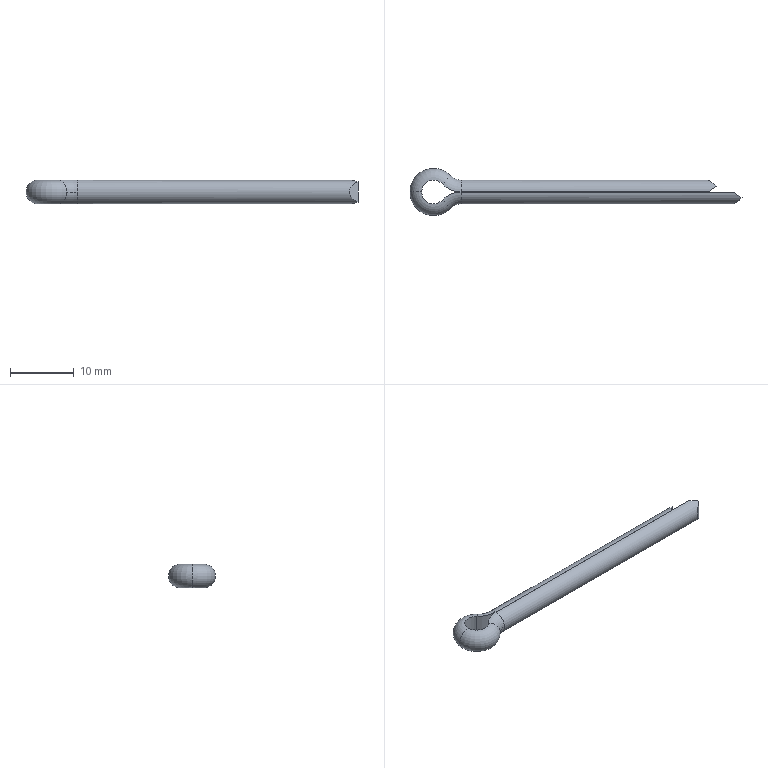Part | SolidWorks | features ICE 1, Sweep 1 | 1 solid | 17 faces | box 52 x 7.4 x 3.7 mm | volume 537.554 mm3 | torus 6 | plane 6 | cylinder 5 | commonest cylinder face diameters 3.7 x2 8.125 x2 3.72 x1
STEP:
#1=CARTESIAN_POINT('',(4.3,0.01,1.85));
#2=VERTEX_POINT('',#1);
#3=CARTESIAN_POINT('',(4.3,1.85,0.));
#4=VERTEX_POINT('',#3);
#5=CARTESIAN_POINT('',(4.3,0.,0.));
#6=DIRECTION('',(-1.,0.,0.));
#7=DIRECTION('',(0.,0.,1.));
#8=AXIS2_PLACEMENT_3D('',#5,#6,#7);
#9=CIRCLE('',#8,1.85);
#10=EDGE_CURVE('',#2,#4,#9,.T.);
#11=ORIENTED_EDGE('',*,*,#10,.T.);
#12=CARTESIAN_POINT('',(2.686,2.544,0.));
#13=VERTEX_POINT('',#12);
#14=CARTESIAN_POINT('',(4.3,4.072,0.));
#15=DIRECTION('',(0.,0.,-1.));
#16=DIRECTION('',(-1.,0.,0.));
#17=AXIS2_PLACEMENT_3D('',#14,#15,#16);
#18=CIRCLE('',#17,2.222);
#19=EDGE_CURVE('',#4,#13,#18,.T.);
#20=ORIENTED_EDGE('',*,*,#19,.T.);
#21=CARTESIAN_POINT('',(1.35,1.279,1.85));
#22=VERTEX_POINT('',#21);
#23=CARTESIAN_POINT('',(1.343,1.272,0.));
#24=DIRECTION('',(-0.6876,0.7261,0.));
#25=DIRECTION('',(0.,0.,1.));
#26=AXIS2_PLACEMENT_3D('',#23,#24,#25);
#27=CIRCLE('',#26,1.85);
#28=EDGE_CURVE('',#22,#13,#27,.T.);
#29=ORIENTED_EDGE('',*,*,#28,.F.);
#30=CARTESIAN_POINT('',(4.3,4.072,1.85));
#31=DIRECTION('',(0.,0.,-1.));
#32=DIRECTION('',(-1.,0.,0.));
#33=AXIS2_PLACEMENT_3D('',#30,#31,#32);
#34=CIRCLE('',#33,4.062);
#35=EDGE_CURVE('',#2,#22,#34,.T.);
#36=ORIENTED_EDGE('',*,*,#35,.F.);
#37=EDGE_LOOP('',(#11,#20,#29,#36));
#38=FACE_OUTER_BOUND('',#37,.T.);
#39=CARTESIAN_POINT('',(4.3,4.072,0.));
#40=DIRECTION('',(0.,0.,-1.));
#41=DIRECTION('',(-1.,0.,0.));
#42=AXIS2_PLACEMENT_3D('',#39,#40,#41);
#43=TOROIDAL_SURFACE('',#42,4.072,1.85);
#44=ADVANCED_FACE('',(#38),#43,.T.);
#45=CARTESIAN_POINT('',(1.35,-1.279,1.85));
#46=VERTEX_POINT('',#45);
#47=CARTESIAN_POINT('',(2.686,-2.544,0.));
#48=VERTEX_POINT('',#47);
#49=CARTESIAN_POINT('',(1.343,-1.272,0.));
#50=DIRECTION('',(0.6876,0.7261,0.));
#51=DIRECTION('',(0.,0.,1.));
#52=AXIS2_PLACEMENT_3D('',#49,#50,#51);
#53=CIRCLE('',#52,1.85);
#54=EDGE_CURVE('',#46,#48,#53,.T.);
#55=ORIENTED_EDGE('',*,*,#54,.T.);
#56=CARTESIAN_POINT('',(4.3,-1.85,0.));
#57=VERTEX_POINT('',#56);
#58=CARTESIAN_POINT('',(4.3,-4.072,0.));
#59=DIRECTION('',(0.,0.,-1.));
#60=DIRECTION('',(-1.,0.,0.));
#61=AXIS2_PLACEMENT_3D('',#58,#59,#60);
#62=CIRCLE('',#61,2.222);
#63=EDGE_CURVE('',#48,#57,#62,.T.);
#64=ORIENTED_EDGE('',*,*,#63,.T.);
#65=CARTESIAN_POINT('',(4.3,-0.01,1.85));
#66=VERTEX_POINT('',#65);
#67=CARTESIAN_POINT('',(4.3,0.,0.));
#68=DIRECTION('',(1.,0.,0.));
#69=DIRECTION('',(0.,0.,1.));
#70=AXIS2_PLACEMENT_3D('',#67,#68,#69);
#71=CIRCLE('',#70,1.85);
#72=EDGE_CURVE('',#66,#57,#71,.T.);
#73=ORIENTED_EDGE('',*,*,#72,.F.);
#74=CARTESIAN_POINT('',(4.3,-4.072,1.85));
#75=DIRECTION('',(0.,0.,-1.));
#76=DIRECTION('',(-1.,0.,0.));
#77=AXIS2_PLACEMENT_3D('',#74,#75,#76);
#78=CIRCLE('',#77,4.062);
#79=EDGE_CURVE('',#46,#66,#78,.T.);
#80=ORIENTED_EDGE('',*,*,#79,.F.);
#81=EDGE_LOOP('',(#55,#64,#73,#80));
#82=FACE_OUTER_BOUND('',#81,.T.);
#83=CARTESIAN_POINT('',(4.3,-4.072,0.));
#84=DIRECTION('',(0.,0.,-1.));
#85=DIRECTION('',(-1.,0.,0.));
#86=AXIS2_PLACEMENT_3D('',#83,#84,#85);
#87=TOROIDAL_SURFACE('',#86,4.072,1.85);
#88=ADVANCED_FACE('',(#82),#87,.T.);
#89=CARTESIAN_POINT('',(1.35,1.279,-1.85));
#90=VERTEX_POINT('',#89);
#91=CARTESIAN_POINT('',(-1.86,0.,-1.85));
#92=VERTEX_POINT('',#91);
#93=CARTESIAN_POINT('',(0.,0.,-1.85));
#94=DIRECTION('',(0.,0.,1.));
#95=DIRECTION('',(1.,0.,0.));
#96=AXIS2_PLACEMENT_3D('',#93,#94,#95);
#97=CIRCLE('',#96,1.86);
#98=EDGE_CURVE('',#90,#92,#97,.T.);
#99=ORIENTED_EDGE('',*,*,#98,.T.);
#100=CARTESIAN_POINT('',(-1.86,0.,1.85));
#101=VERTEX_POINT('',#100);
#102=CARTESIAN_POINT('',(-1.85,0.,0.));
#103=DIRECTION('',(0.,1.,0.));
#104=DIRECTION('',(-1.,0.,0.));
#105=AXIS2_PLACEMENT_3D('',#102,#103,#104);
#106=CIRCLE('',#105,1.85);
#107=EDGE_CURVE('',#92,#101,#106,.T.);
#108=ORIENTED_EDGE('',*,*,#107,.T.);
#109=CARTESIAN_POINT('',(0.,0.,1.85));
#110=DIRECTION('',(0.,0.,1.));
#111=DIRECTION('',(1.,0.,0.));
#112=AXIS2_PLACEMENT_3D('',#109,#110,#111);
#113=CIRCLE('',#112,1.86);
#114=EDGE_CURVE('',#22,#101,#113,.T.);
#115=ORIENTED_EDGE('',*,*,#114,.F.);
#116=ORIENTED_EDGE('',*,*,#28,.T.);
#117=CARTESIAN_POINT('',(1.343,1.272,0.));
#118=DIRECTION('',(-0.6876,0.7261,0.));
#119=DIRECTION('',(0.,0.,1.));
#120=AXIS2_PLACEMENT_3D('',#117,#118,#119);
#121=CIRCLE('',#120,1.85);
#122=EDGE_CURVE('',#13,#90,#121,.T.);
#123=ORIENTED_EDGE('',*,*,#122,.T.);
#124=EDGE_LOOP('',(#99,#108,#115,#116,#123));
#125=FACE_OUTER_BOUND('',#124,.T.);
#126=CARTESIAN_POINT('',(0.,0.,0.));
#127=DIRECTION('',(0.,0.,1.));
#128=DIRECTION('',(1.,0.,0.));
#129=AXIS2_PLACEMENT_3D('',#126,#127,#128);
#130=TOROIDAL_SURFACE('',#129,1.85,1.85);
#131=ADVANCED_FACE('',(#125),#130,.T.);
#132=CARTESIAN_POINT('',(48.3,-0.93,-1.599));
#133=VERTEX_POINT('',#132);
#134=CARTESIAN_POINT('',(46.997,-0.01,-1.85));
#135=VERTEX_POINT('',#134);
#136=CARTESIAN_POINT('',(48.3,-0.93,-1.599));
#137=CARTESIAN_POINT('',(47.902,-0.6489,-1.763));
#138=CARTESIAN_POINT('',(47.457,-0.3352,-1.848));
#139=CARTESIAN_POINT('',(46.997,-0.01,-1.85));
#140=(BOUNDED_CURVE()B_SPLINE_CURVE(3,(#136,#137,#138,#139),.UNSPECIFIED.,.F.,.F.)B_SPLINE_CURVE_WITH_KNOTS((4,4),(1.044,1.565),.UNSPECIFIED.)CURVE()GEOMETRIC_REPRESENTATION_ITEM()RATIONAL_B_SPLINE_CURVE((1.,0.9775,0.9775,1.))REPRESENTATION_ITEM(''));
#141=EDGE_CURVE('',#133,#135,#140,.T.);
#142=ORIENTED_EDGE('',*,*,#141,.F.);
#143=CARTESIAN_POINT('',(48.3,-0.93,1.599));
#144=VERTEX_POINT('',#143);
#145=CARTESIAN_POINT('',(48.3,-0.93,1.599));
#146=CARTESIAN_POINT('',(46.315,-2.309,0.7975));
#147=CARTESIAN_POINT('',(46.315,-2.309,-0.7975));
#148=CARTESIAN_POINT('',(48.3,-0.93,-1.599));
#149=(BOUNDED_CURVE()B_SPLINE_CURVE(3,(#145,#146,#147,#148),.UNSPECIFIED.,.F.,.T.)B_SPLINE_CURVE_WITH_KNOTS((4,4),(2.098,4.186),.UNSPECIFIED.)CURVE()GEOMETRIC_REPRESENTATION_ITEM()RATIONAL_B_SPLINE_CURVE((1.,0.6685,0.6685,1.))REPRESENTATION_ITEM(''));
#150=EDGE_CURVE('',#144,#133,#149,.T.);
#151=ORIENTED_EDGE('',*,*,#150,.F.);
#152=CARTESIAN_POINT('',(46.997,-0.01,1.85));
#153=VERTEX_POINT('',#152);
#154=CARTESIAN_POINT('',(46.997,-0.01,1.85));
#155=CARTESIAN_POINT('',(47.457,-0.3352,1.848));
#156=CARTESIAN_POINT('',(47.902,-0.6489,1.763));
#157=CARTESIAN_POINT('',(48.3,-0.93,1.599));
#158=(BOUNDED_CURVE()B_SPLINE_CURVE(3,(#154,#155,#156,#157),.UNSPECIFIED.,.F.,.T.)B_SPLINE_CURVE_WITH_KNOTS((4,4),(4.718,5.239),.UNSPECIFIED.)CURVE()GEOMETRIC_REPRESENTATION_ITEM()RATIONAL_B_SPLINE_CURVE((1.,0.9775,0.9775,1.))REPRESENTATION_ITEM(''));
#159=EDGE_CURVE('',#153,#144,#158,.T.);
#160=ORIENTED_EDGE('',*,*,#159,.F.);
#161=CARTESIAN_POINT('',(4.3,-0.01,1.85));
#162=DIRECTION('',(1.,0.,0.));
#163=VECTOR('',#162,1000.);
#164=LINE('',#161,#163);
#165=EDGE_CURVE('',#66,#153,#164,.T.);
#166=ORIENTED_EDGE('',*,*,#165,.F.);
#167=ORIENTED_EDGE('',*,*,#72,.T.);
#168=CARTESIAN_POINT('',(4.3,-0.01,-1.85));
#169=VERTEX_POINT('',#168);
#170=CARTESIAN_POINT('',(4.3,0.,0.));
#171=DIRECTION('',(1.,0.,0.));
#172=DIRECTION('',(0.,0.,1.));
#173=AXIS2_PLACEMENT_3D('',#170,#171,#172);
#174=CIRCLE('',#173,1.85);
#175=EDGE_CURVE('',#57,#169,#174,.T.);
#176=ORIENTED_EDGE('',*,*,#175,.T.);
#177=CARTESIAN_POINT('',(4.3,-0.01,-1.85));
#178=DIRECTION('',(1.,0.,0.));
#179=VECTOR('',#178,1000.);
#180=LINE('',#177,#179);
#181=EDGE_CURVE('',#169,#135,#180,.T.);
#182=ORIENTED_EDGE('',*,*,#181,.T.);
#183=EDGE_LOOP('',(#142,#151,#160,#166,#167,#176,#182));
#184=FACE_OUTER_BOUND('',#183,.T.);
#185=CARTESIAN_POINT('',(4.3,0.,0.));
#186=DIRECTION('',(1.,0.,0.));
#187=DIRECTION('',(0.,0.,-1.));
#188=AXIS2_PLACEMENT_3D('',#185,#186,#187);
#189=CYLINDRICAL_SURFACE('',#188,1.85);
#190=ADVANCED_FACE('',(#184),#189,.T.);
#191=CARTESIAN_POINT('',(46.997,-0.01,-1.85));
#192=DIRECTION('',(0.,0.,1.));
#193=VECTOR('',#192,1000.);
#194=LINE('',#191,#193);
#195=EDGE_CURVE('',#135,#153,#194,.T.);
#196=ORIENTED_EDGE('',*,*,#195,.F.);
#197=ORIENTED_EDGE('',*,*,#181,.F.);
#198=CARTESIAN_POINT('',(4.3,-0.01,-1.85));
#199=DIRECTION('',(0.,0.,1.));
#200=VECTOR('',#199,1000.);
#201=LINE('',#198,#200);
#202=EDGE_CURVE('',#169,#66,#201,.T.);
#203=ORIENTED_EDGE('',*,*,#202,.T.);
#204=ORIENTED_EDGE('',*,*,#165,.T.);
#205=EDGE_LOOP('',(#196,#197,#203,#204));
#206=FACE_OUTER_BOUND('',#205,.T.);
#207=CARTESIAN_POINT('',(4.3,-0.01,-1.85));
#208=DIRECTION('',(0.,1.,0.));
#209=DIRECTION('',(0.,0.,1.));
#210=AXIS2_PLACEMENT_3D('',#207,#208,#209);
#211=PLANE('',#210);
#212=ADVANCED_FACE('',(#206),#211,.T.);
#213=CARTESIAN_POINT('',(1.35,-1.279,-1.85));
#214=VERTEX_POINT('',#213);
#215=CARTESIAN_POINT('',(1.35,-1.279,-1.85));
#216=DIRECTION('',(0.,0.,1.));
#217=VECTOR('',#216,1000.);
#218=LINE('',#215,#217);
#219=EDGE_CURVE('',#214,#46,#218,.T.);
#220=ORIENTED_EDGE('',*,*,#219,.T.);
#221=ORIENTED_EDGE('',*,*,#79,.T.);
#222=ORIENTED_EDGE('',*,*,#202,.F.);
#223=CARTESIAN_POINT('',(4.3,-4.072,-1.85));
#224=DIRECTION('',(0.,0.,-1.));
#225=DIRECTION('',(-1.,0.,0.));
#226=AXIS2_PLACEMENT_3D('',#223,#224,#225);
#227=CIRCLE('',#226,4.062);
#228=EDGE_CURVE('',#214,#169,#227,.T.);
#229=ORIENTED_EDGE('',*,*,#228,.F.);
#230=EDGE_LOOP('',(#220,#221,#222,#229));
#231=FACE_OUTER_BOUND('',#230,.T.);
#232=CARTESIAN_POINT('',(4.3,-4.072,0.));
#233=DIRECTION('',(0.,0.,-1.));
#234=DIRECTION('',(-1.,0.,0.));
#235=AXIS2_PLACEMENT_3D('',#232,#233,#234);
#236=CYLINDRICAL_SURFACE('',#235,4.062);
#237=ADVANCED_FACE('',(#231),#236,.T.);
#238=ORIENTED_EDGE('',*,*,#63,.F.);
#239=CARTESIAN_POINT('',(1.343,-1.272,0.));
#240=DIRECTION('',(0.6876,0.7261,0.));
#241=DIRECTION('',(0.,0.,1.));
#242=AXIS2_PLACEMENT_3D('',#239,#240,#241);
#243=CIRCLE('',#242,1.85);
#244=EDGE_CURVE('',#48,#214,#243,.T.);
#245=ORIENTED_EDGE('',*,*,#244,.T.);
#246=ORIENTED_EDGE('',*,*,#228,.T.);
#247=ORIENTED_EDGE('',*,*,#175,.F.);
#248=EDGE_LOOP('',(#238,#245,#246,#247));
#249=FACE_OUTER_BOUND('',#248,.T.);
#250=CARTESIAN_POINT('',(4.3,-4.072,0.));
#251=DIRECTION('',(0.,0.,-1.));
#252=DIRECTION('',(-1.,0.,0.));
#253=AXIS2_PLACEMENT_3D('',#250,#251,#252);
#254=TOROIDAL_SURFACE('',#253,4.072,1.85);
#255=ADVANCED_FACE('',(#249),#254,.T.);
#256=CARTESIAN_POINT('',(1.35,1.279,-1.85));
#257=DIRECTION('',(0.,0.,1.));
#258=VECTOR('',#257,1000.);
#259=LINE('',#256,#258);
#260=EDGE_CURVE('',#90,#22,#259,.T.);
#261=ORIENTED_EDGE('',*,*,#260,.T.);
#262=ORIENTED_EDGE('',*,*,#114,.T.);
#263=CARTESIAN_POINT('',(0.,0.,1.85));
#264=DIRECTION('',(0.,0.,1.));
#265=DIRECTION('',(1.,0.,0.));
#266=AXIS2_PLACEMENT_3D('',#263,#264,#265);
#267=CIRCLE('',#266,1.86);
#268=EDGE_CURVE('',#101,#46,#267,.T.);
#269=ORIENTED_EDGE('',*,*,#268,.T.);
#270=ORIENTED_EDGE('',*,*,#219,.F.);
#271=CARTESIAN_POINT('',(0.,0.,-1.85));
#272=DIRECTION('',(0.,0.,1.));
#273=DIRECTION('',(1.,0.,0.));
#274=AXIS2_PLACEMENT_3D('',#271,#272,#273);
#275=CIRCLE('',#274,1.86);
#276=EDGE_CURVE('',#92,#214,#275,.T.);
#277=ORIENTED_EDGE('',*,*,#276,.F.);
#278=ORIENTED_EDGE('',*,*,#98,.F.);
#279=EDGE_LOOP('',(#261,#262,#269,#270,#277,#278));
#280=FACE_OUTER_BOUND('',#279,.T.);
#281=CARTESIAN_POINT('',(0.,0.,0.));
#282=DIRECTION('',(0.,0.,1.));
#283=DIRECTION('',(1.,0.,0.));
#284=AXIS2_PLACEMENT_3D('',#281,#282,#283);
#285=CYLINDRICAL_SURFACE('',#284,1.86);
#286=ADVANCED_FACE('',(#280),#285,.F.);
#287=ORIENTED_EDGE('',*,*,#107,.F.);
#288=ORIENTED_EDGE('',*,*,#276,.T.);
#289=ORIENTED_EDGE('',*,*,#244,.F.);
#290=ORIENTED_EDGE('',*,*,#54,.F.);
#291=ORIENTED_EDGE('',*,*,#268,.F.);
#292=EDGE_LOOP('',(#287,#288,#289,#290,#291));
#293=FACE_OUTER_BOUND('',#292,.T.);
#294=CARTESIAN_POINT('',(0.,0.,0.));
#295=DIRECTION('',(0.,0.,1.));
#296=DIRECTION('',(1.,0.,0.));
#297=AXIS2_PLACEMENT_3D('',#294,#295,#296);
#298=TOROIDAL_SURFACE('',#297,1.85,1.85);
#299=ADVANCED_FACE('',(#293),#298,.T.);
#300=CARTESIAN_POINT('',(4.3,0.01,-1.85));
#301=VERTEX_POINT('',#300);
#302=CARTESIAN_POINT('',(4.3,0.01,-1.85));
#303=DIRECTION('',(0.,0.,1.));
#304=VECTOR('',#303,1000.);
#305=LINE('',#302,#304);
#306=EDGE_CURVE('',#301,#2,#305,.T.);
#307=ORIENTED_EDGE('',*,*,#306,.T.);
#308=ORIENTED_EDGE('',*,*,#35,.T.);
#309=ORIENTED_EDGE('',*,*,#260,.F.);
#310=CARTESIAN_POINT('',(4.3,4.072,-1.85));
#311=DIRECTION('',(0.,0.,-1.));
#312=DIRECTION('',(-1.,0.,0.));
#313=AXIS2_PLACEMENT_3D('',#310,#311,#312);
#314=CIRCLE('',#313,4.062);
#315=EDGE_CURVE('',#301,#90,#314,.T.);
#316=ORIENTED_EDGE('',*,*,#315,.F.);
#317=EDGE_LOOP('',(#307,#308,#309,#316));
#318=FACE_OUTER_BOUND('',#317,.T.);
#319=CARTESIAN_POINT('',(4.3,4.072,0.));
#320=DIRECTION('',(0.,0.,-1.));
#321=DIRECTION('',(-1.,0.,0.));
#322=AXIS2_PLACEMENT_3D('',#319,#320,#321);
#323=CYLINDRICAL_SURFACE('',#322,4.062);
#324=ADVANCED_FACE('',(#318),#323,.T.);
#325=ORIENTED_EDGE('',*,*,#19,.F.);
#326=CARTESIAN_POINT('',(4.3,0.,0.));
#327=DIRECTION('',(-1.,0.,0.));
#328=DIRECTION('',(0.,0.,1.));
#329=AXIS2_PLACEMENT_3D('',#326,#327,#328);
#330=CIRCLE('',#329,1.85);
#331=EDGE_CURVE('',#4,#301,#330,.T.);
#332=ORIENTED_EDGE('',*,*,#331,.T.);
#333=ORIENTED_EDGE('',*,*,#315,.T.);
#334=ORIENTED_EDGE('',*,*,#122,.F.);
#335=EDGE_LOOP('',(#325,#332,#333,#334));
#336=FACE_OUTER_BOUND('',#335,.T.);
#337=CARTESIAN_POINT('',(4.3,4.072,0.));
#338=DIRECTION('',(0.,0.,-1.));
#339=DIRECTION('',(-1.,0.,0.));
#340=AXIS2_PLACEMENT_3D('',#337,#338,#339);
#341=TOROIDAL_SURFACE('',#340,4.072,1.85);
#342=ADVANCED_FACE('',(#336),#341,.T.);
#343=CARTESIAN_POINT('',(42.99,0.01,1.85));
#344=VERTEX_POINT('',#343);
#345=CARTESIAN_POINT('',(4.3,0.01,1.85));
#346=DIRECTION('',(1.,0.,0.));
#347=VECTOR('',#346,1000.);
#348=LINE('',#345,#347);
#349=EDGE_CURVE('',#2,#344,#348,.T.);
#350=ORIENTED_EDGE('',*,*,#349,.T.);
#351=CARTESIAN_POINT('',(44.3,0.92,1.605));
#352=VERTEX_POINT('',#351);
#353=CARTESIAN_POINT('',(42.99,0.01,1.85));
#354=CARTESIAN_POINT('',(43.452,0.3312,1.848));
#355=CARTESIAN_POINT('',(43.899,0.6413,1.765));
#356=CARTESIAN_POINT('',(44.3,0.92,1.605));
#357=(BOUNDED_CURVE()B_SPLINE_CURVE(3,(#353,#354,#355,#356),.UNSPECIFIED.,.F.,.T.)B_SPLINE_CURVE_WITH_KNOTS((4,4),(4.718,5.233),.UNSPECIFIED.)CURVE()GEOMETRIC_REPRESENTATION_ITEM()RATIONAL_B_SPLINE_CURVE((1.,0.978,0.978,1.))REPRESENTATION_ITEM(''));
#358=EDGE_CURVE('',#344,#352,#357,.T.);
#359=ORIENTED_EDGE('',*,*,#358,.T.);
#360=CARTESIAN_POINT('',(44.3,0.92,-1.605));
#361=VERTEX_POINT('',#360);
#362=CARTESIAN_POINT('',(44.3,0.92,1.605));
#363=CARTESIAN_POINT('',(42.322,2.316,0.8047));
#364=CARTESIAN_POINT('',(42.322,2.316,-0.8047));
#365=CARTESIAN_POINT('',(44.3,0.92,-1.605));
#366=(BOUNDED_CURVE()B_SPLINE_CURVE(3,(#362,#363,#364,#365),.UNSPECIFIED.,.F.,.F.)B_SPLINE_CURVE_WITH_KNOTS((4,4),(2.091,4.192),.UNSPECIFIED.)CURVE()GEOMETRIC_REPRESENTATION_ITEM()RATIONAL_B_SPLINE_CURVE((1.,0.6649,0.6649,1.))REPRESENTATION_ITEM(''));
#367=EDGE_CURVE('',#352,#361,#366,.T.);
#368=ORIENTED_EDGE('',*,*,#367,.T.);
#369=CARTESIAN_POINT('',(42.99,0.01,-1.85));
#370=VERTEX_POINT('',#369);
#371=CARTESIAN_POINT('',(44.3,0.92,-1.605));
#372=CARTESIAN_POINT('',(43.899,0.6413,-1.765));
#373=CARTESIAN_POINT('',(43.452,0.3312,-1.848));
#374=CARTESIAN_POINT('',(42.99,0.01,-1.85));
#375=(BOUNDED_CURVE()B_SPLINE_CURVE(3,(#371,#372,#373,#374),.UNSPECIFIED.,.F.,.F.)B_SPLINE_CURVE_WITH_KNOTS((4,4),(1.05,1.565),.UNSPECIFIED.)CURVE()GEOMETRIC_REPRESENTATION_ITEM()RATIONAL_B_SPLINE_CURVE((1.,0.978,0.978,1.))REPRESENTATION_ITEM(''));
#376=EDGE_CURVE('',#361,#370,#375,.T.);
#377=ORIENTED_EDGE('',*,*,#376,.T.);
#378=CARTESIAN_POINT('',(4.3,0.01,-1.85));
#379=DIRECTION('',(1.,0.,0.));
#380=VECTOR('',#379,1000.);
#381=LINE('',#378,#380);
#382=EDGE_CURVE('',#301,#370,#381,.T.);
#383=ORIENTED_EDGE('',*,*,#382,.F.);
#384=ORIENTED_EDGE('',*,*,#331,.F.);
#385=ORIENTED_EDGE('',*,*,#10,.F.);
#386=EDGE_LOOP('',(#350,#359,#368,#377,#383,#384,#385));
#387=FACE_OUTER_BOUND('',#386,.T.);
#388=CARTESIAN_POINT('',(4.3,0.,0.));
#389=DIRECTION('',(1.,0.,0.));
#390=DIRECTION('',(0.,0.,-1.));
#391=AXIS2_PLACEMENT_3D('',#388,#389,#390);
#392=CYLINDRICAL_SURFACE('',#391,1.85);
#393=ADVANCED_FACE('',(#387),#392,.T.);
#394=ORIENTED_EDGE('',*,*,#382,.T.);
#395=CARTESIAN_POINT('',(42.99,0.01,-1.85));
#396=DIRECTION('',(0.,0.,1.));
#397=VECTOR('',#396,1000.);
#398=LINE('',#395,#397);
#399=EDGE_CURVE('',#370,#344,#398,.T.);
#400=ORIENTED_EDGE('',*,*,#399,.T.);
#401=ORIENTED_EDGE('',*,*,#349,.F.);
#402=ORIENTED_EDGE('',*,*,#306,.F.);
#403=EDGE_LOOP('',(#394,#400,#401,#402));
#404=FACE_OUTER_BOUND('',#403,.T.);
#405=CARTESIAN_POINT('',(4.3,0.01,-1.85));
#406=DIRECTION('',(0.,1.,0.));
#407=DIRECTION('',(0.,0.,1.));
#408=AXIS2_PLACEMENT_3D('',#405,#406,#407);
#409=PLANE('',#408);
#410=ADVANCED_FACE('',(#404),#409,.F.);
#411=CARTESIAN_POINT('',(44.3,0.92,-1.85));
#412=DIRECTION('',(0.,0.,1.));
#413=VECTOR('',#412,1000.);
#414=LINE('',#411,#413);
#415=EDGE_CURVE('',#361,#352,#414,.T.);
#416=ORIENTED_EDGE('',*,*,#415,.T.);
#417=ORIENTED_EDGE('',*,*,#358,.F.);
#418=ORIENTED_EDGE('',*,*,#399,.F.);
#419=ORIENTED_EDGE('',*,*,#376,.F.);
#420=EDGE_LOOP('',(#416,#417,#418,#419));
#421=FACE_OUTER_BOUND('',#420,.T.);
#422=CARTESIAN_POINT('',(44.3,0.92,-1.85));
#423=DIRECTION('',(-0.5705,0.8213,0.));
#424=DIRECTION('',(-0.8213,-0.5705,0.));
#425=AXIS2_PLACEMENT_3D('',#422,#423,#424);
#426=PLANE('',#425);
#427=ADVANCED_FACE('',(#421),#426,.F.);
#428=ORIENTED_EDGE('',*,*,#415,.F.);
#429=ORIENTED_EDGE('',*,*,#367,.F.);
#430=EDGE_LOOP('',(#428,#429));
#431=FACE_OUTER_BOUND('',#430,.T.);
#432=CARTESIAN_POINT('',(44.3,0.92,-1.85));
#433=DIRECTION('',(-0.5767,-0.817,0.));
#434=DIRECTION('',(0.817,-0.5767,0.));
#435=AXIS2_PLACEMENT_3D('',#432,#433,#434);
#436=PLANE('',#435);
#437=ADVANCED_FACE('',(#431),#436,.F.);
#438=ORIENTED_EDGE('',*,*,#150,.T.);
#439=CARTESIAN_POINT('',(48.3,-0.93,-1.85));
#440=DIRECTION('',(0.,0.,1.));
#441=VECTOR('',#440,1000.);
#442=LINE('',#439,#441);
#443=EDGE_CURVE('',#133,#144,#442,.T.);
#444=ORIENTED_EDGE('',*,*,#443,.T.);
#445=EDGE_LOOP('',(#438,#444));
#446=FACE_OUTER_BOUND('',#445,.T.);
#447=CARTESIAN_POINT('',(48.3,-0.93,-1.85));
#448=DIRECTION('',(-0.5705,0.8213,0.));
#449=DIRECTION('',(-0.8213,-0.5705,0.));
#450=AXIS2_PLACEMENT_3D('',#447,#448,#449);
#451=PLANE('',#450);
#452=ADVANCED_FACE('',(#446),#451,.F.);
#453=ORIENTED_EDGE('',*,*,#141,.T.);
#454=ORIENTED_EDGE('',*,*,#195,.T.);
#455=ORIENTED_EDGE('',*,*,#159,.T.);
#456=ORIENTED_EDGE('',*,*,#443,.F.);
#457=EDGE_LOOP('',(#453,#454,#455,#456));
#458=FACE_OUTER_BOUND('',#457,.T.);
#459=CARTESIAN_POINT('',(48.3,-0.93,-1.85));
#460=DIRECTION('',(-0.5767,-0.817,0.));
#461=DIRECTION('',(0.817,-0.5767,0.));
#462=AXIS2_PLACEMENT_3D('',#459,#460,#461);
#463=PLANE('',#462);
#464=ADVANCED_FACE('',(#458),#463,.F.);
#465=CLOSED_SHELL('',(#44,#88,#131,#190,#212,#237,#255,#286,#299,#324,#342,#393,#410,#427,#437,#452,#464));
#466=MANIFOLD_SOLID_BREP('',#465);
#467=CARTESIAN_POINT('',(0.,0.,0.));
#468=DIRECTION('',(0.,0.,1.));
#469=DIRECTION('',(1.,0.,0.));
#470=AXIS2_PLACEMENT_3D('',#467,#468,#469);
#471=(LENGTH_UNIT()NAMED_UNIT(*)SI_UNIT(.MILLI.,.METRE.));
#472=UNCERTAINTY_MEASURE_WITH_UNIT(LENGTH_MEASURE(0.00001),#471,'','');
#473=(NAMED_UNIT(*)PLANE_ANGLE_UNIT()SI_UNIT($,.RADIAN.));
#474=(NAMED_UNIT(*)SI_UNIT($,.STERADIAN.)SOLID_ANGLE_UNIT());
#475=(GEOMETRIC_REPRESENTATION_CONTEXT(3)GLOBAL_UNCERTAINTY_ASSIGNED_CONTEXT((#472))GLOBAL_UNIT_ASSIGNED_CONTEXT((#471,#473,#474))REPRESENTATION_CONTEXT('',''));
#476=ADVANCED_BREP_SHAPE_REPRESENTATION('',(#466,#470),#475);